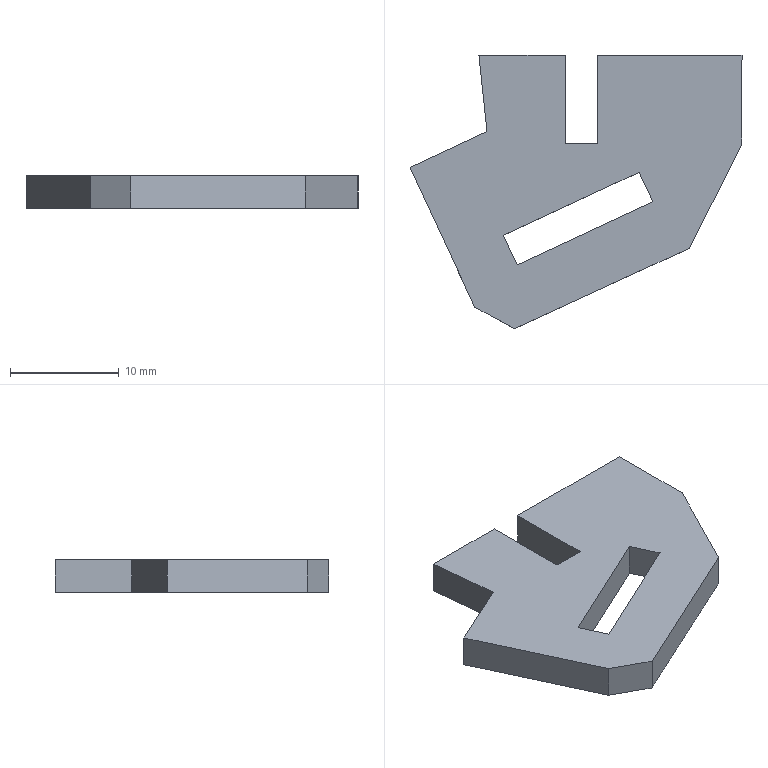Part | SolidWorks | features BaseBody 1 | 1 solid | 18 faces | box 30.485 x 25.117 x 3 mm | volume 1409 mm3 | plane 18
STEP:
#1=CARTESIAN_POINT('',(16.164,-13.547,-1.5));
#2=VERTEX_POINT('',#1);
#3=CARTESIAN_POINT('',(14.9,-10.831,-1.5));
#4=VERTEX_POINT('',#3);
#5=CARTESIAN_POINT('',(8.106,3.772,-1.5));
#6=DIRECTION('',(-0.4219,0.9067,0.));
#7=VECTOR('',#6,1000.);
#8=LINE('',#5,#7);
#9=EDGE_CURVE('',#2,#4,#8,.T.);
#10=ORIENTED_EDGE('',*,*,#9,.T.);
#11=CARTESIAN_POINT('',(2.431,-16.623,-1.5));
#12=VERTEX_POINT('',#11);
#13=CARTESIAN_POINT('',(6.783,-14.601,-1.5));
#14=DIRECTION('',(-0.9069,-0.4213,0.));
#15=VECTOR('',#14,1000.);
#16=LINE('',#13,#15);
#17=EDGE_CURVE('',#4,#12,#16,.T.);
#18=ORIENTED_EDGE('',*,*,#17,.T.);
#19=CARTESIAN_POINT('',(3.694,-19.34,-1.5));
#20=VERTEX_POINT('',#19);
#21=CARTESIAN_POINT('',(-4.353,-2.023,-1.5));
#22=DIRECTION('',(0.4214,-0.9069,0.));
#23=VECTOR('',#22,1000.);
#24=LINE('',#21,#23);
#25=EDGE_CURVE('',#12,#20,#24,.T.);
#26=ORIENTED_EDGE('',*,*,#25,.T.);
#27=CARTESIAN_POINT('',(8.045,-17.318,-1.5));
#28=DIRECTION('',(0.9069,0.4213,0.));
#29=VECTOR('',#28,1000.);
#30=LINE('',#27,#29);
#31=EDGE_CURVE('',#20,#2,#30,.T.);
#32=ORIENTED_EDGE('',*,*,#31,.T.);
#33=EDGE_LOOP('',(#10,#18,#26,#32));
#34=FACE_BOUND('',#33,.T.);
#35=CARTESIAN_POINT('',(19.491,-17.818,-1.5));
#36=VERTEX_POINT('',#35);
#37=CARTESIAN_POINT('',(24.349,-8.242,-1.5));
#38=VERTEX_POINT('',#37);
#39=CARTESIAN_POINT('',(22.69,-11.511,-1.5));
#40=DIRECTION('',(0.4524,0.8918,0.));
#41=VECTOR('',#40,1000.);
#42=LINE('',#39,#41);
#43=EDGE_CURVE('',#36,#38,#42,.T.);
#44=ORIENTED_EDGE('',*,*,#43,.F.);
#45=CARTESIAN_POINT('',(3.466,-25.2,-1.5));
#46=VERTEX_POINT('',#45);
#47=CARTESIAN_POINT('',(10.184,-22.105,-1.5));
#48=DIRECTION('',(0.9083,0.4184,0.));
#49=VECTOR('',#48,1000.);
#50=LINE('',#47,#49);
#51=EDGE_CURVE('',#46,#36,#50,.T.);
#52=ORIENTED_EDGE('',*,*,#51,.F.);
#53=CARTESIAN_POINT('',(-0.1829,-23.22,-1.5));
#54=VERTEX_POINT('',#53);
#55=CARTESIAN_POINT('',(-9.776,-18.014,-1.5));
#56=DIRECTION('',(0.8789,-0.477,0.));
#57=VECTOR('',#56,1000.);
#58=LINE('',#55,#57);
#59=EDGE_CURVE('',#54,#46,#58,.T.);
#60=ORIENTED_EDGE('',*,*,#59,.F.);
#61=CARTESIAN_POINT('',(-6.136,-10.378,-1.5));
#62=VERTEX_POINT('',#61);
#63=CARTESIAN_POINT('',(-9.011,-4.177,-1.5));
#64=DIRECTION('',(0.4206,-0.9073,0.));
#65=VECTOR('',#64,1000.);
#66=LINE('',#63,#65);
#67=EDGE_CURVE('',#62,#54,#66,.T.);
#68=ORIENTED_EDGE('',*,*,#67,.F.);
#69=CARTESIAN_POINT('',(0.9311,-7.102,-1.5));
#70=VERTEX_POINT('',#69);
#71=CARTESIAN_POINT('',(2.875,-6.201,-1.5));
#72=DIRECTION('',(-0.9073,-0.4206,0.));
#73=VECTOR('',#72,1000.);
#74=LINE('',#71,#73);
#75=EDGE_CURVE('',#70,#62,#74,.T.);
#76=ORIENTED_EDGE('',*,*,#75,.F.);
#77=CARTESIAN_POINT('',(0.193,-0.08325,-1.5));
#78=VERTEX_POINT('',#77);
#79=CARTESIAN_POINT('',(0.1822,0.01916,-1.5));
#80=DIRECTION('',(0.1046,-0.9945,0.));
#81=VECTOR('',#80,1000.);
#82=LINE('',#79,#81);
#83=EDGE_CURVE('',#78,#70,#82,.T.);
#84=ORIENTED_EDGE('',*,*,#83,.F.);
#85=CARTESIAN_POINT('',(8.101,-0.08325,-1.5));
#86=VERTEX_POINT('',#85);
#87=CARTESIAN_POINT('',(0.,-0.08325,-1.5));
#88=DIRECTION('',(1.,0.,0.));
#89=VECTOR('',#88,1000.);
#90=LINE('',#87,#89);
#91=EDGE_CURVE('',#78,#86,#90,.T.);
#92=ORIENTED_EDGE('',*,*,#91,.T.);
#93=CARTESIAN_POINT('',(8.13,-8.195,-1.5));
#94=VERTEX_POINT('',#93);
#95=CARTESIAN_POINT('',(8.101,0.02877,-1.5));
#96=DIRECTION('',(-0.003551,1.,0.));
#97=VECTOR('',#96,1000.);
#98=LINE('',#95,#97);
#99=EDGE_CURVE('',#94,#86,#98,.T.);
#100=ORIENTED_EDGE('',*,*,#99,.F.);
#101=CARTESIAN_POINT('',(11.126,-8.195,-1.5));
#102=VERTEX_POINT('',#101);
#103=CARTESIAN_POINT('',(0.,-8.195,-1.5));
#104=DIRECTION('',(-1.,0.,0.));
#105=VECTOR('',#104,1000.);
#106=LINE('',#103,#105);
#107=EDGE_CURVE('',#102,#94,#106,.T.);
#108=ORIENTED_EDGE('',*,*,#107,.F.);
#109=CARTESIAN_POINT('',(11.126,-0.08325,-1.5));
#110=VERTEX_POINT('',#109);
#111=CARTESIAN_POINT('',(11.126,0.,-1.5));
#112=DIRECTION('',(0.,-1.,0.));
#113=VECTOR('',#112,1000.);
#114=LINE('',#111,#113);
#115=EDGE_CURVE('',#110,#102,#114,.T.);
#116=ORIENTED_EDGE('',*,*,#115,.F.);
#117=CARTESIAN_POINT('',(24.349,-0.08325,-1.5));
#118=VERTEX_POINT('',#117);
#119=CARTESIAN_POINT('',(0.,-0.08325,-1.5));
#120=DIRECTION('',(1.,0.,0.));
#121=VECTOR('',#120,1000.);
#122=LINE('',#119,#121);
#123=EDGE_CURVE('',#110,#118,#122,.T.);
#124=ORIENTED_EDGE('',*,*,#123,.T.);
#125=CARTESIAN_POINT('',(24.349,0.,-1.5));
#126=DIRECTION('',(0.,1.,0.));
#127=VECTOR('',#126,1000.);
#128=LINE('',#125,#127);
#129=EDGE_CURVE('',#38,#118,#128,.T.);
#130=ORIENTED_EDGE('',*,*,#129,.F.);
#131=EDGE_LOOP('',(#44,#52,#60,#68,#76,#84,#92,#100,#108,#116,#124,#130));
#132=FACE_OUTER_BOUND('',#131,.T.);
#133=CARTESIAN_POINT('',(0.,0.,-1.5));
#134=DIRECTION('',(0.,0.,1.));
#135=DIRECTION('',(1.,0.,0.));
#136=AXIS2_PLACEMENT_3D('',#133,#134,#135);
#137=PLANE('',#136);
#138=ADVANCED_FACE('',(#34,#132),#137,.F.);
#139=CARTESIAN_POINT('',(16.164,-13.547,1.5));
#140=VERTEX_POINT('',#139);
#141=CARTESIAN_POINT('',(14.9,-10.831,1.5));
#142=VERTEX_POINT('',#141);
#143=CARTESIAN_POINT('',(8.106,3.772,1.5));
#144=DIRECTION('',(-0.4219,0.9067,0.));
#145=VECTOR('',#144,1000.);
#146=LINE('',#143,#145);
#147=EDGE_CURVE('',#140,#142,#146,.T.);
#148=ORIENTED_EDGE('',*,*,#147,.F.);
#149=CARTESIAN_POINT('',(3.694,-19.34,1.5));
#150=VERTEX_POINT('',#149);
#151=CARTESIAN_POINT('',(8.045,-17.318,1.5));
#152=DIRECTION('',(0.9069,0.4213,0.));
#153=VECTOR('',#152,1000.);
#154=LINE('',#151,#153);
#155=EDGE_CURVE('',#150,#140,#154,.T.);
#156=ORIENTED_EDGE('',*,*,#155,.F.);
#157=CARTESIAN_POINT('',(2.431,-16.623,1.5));
#158=VERTEX_POINT('',#157);
#159=CARTESIAN_POINT('',(-4.353,-2.023,1.5));
#160=DIRECTION('',(0.4214,-0.9069,0.));
#161=VECTOR('',#160,1000.);
#162=LINE('',#159,#161);
#163=EDGE_CURVE('',#158,#150,#162,.T.);
#164=ORIENTED_EDGE('',*,*,#163,.F.);
#165=CARTESIAN_POINT('',(6.783,-14.601,1.5));
#166=DIRECTION('',(-0.9069,-0.4213,0.));
#167=VECTOR('',#166,1000.);
#168=LINE('',#165,#167);
#169=EDGE_CURVE('',#142,#158,#168,.T.);
#170=ORIENTED_EDGE('',*,*,#169,.F.);
#171=EDGE_LOOP('',(#148,#156,#164,#170));
#172=FACE_BOUND('',#171,.T.);
#173=CARTESIAN_POINT('',(19.491,-17.818,1.5));
#174=VERTEX_POINT('',#173);
#175=CARTESIAN_POINT('',(24.349,-8.242,1.5));
#176=VERTEX_POINT('',#175);
#177=CARTESIAN_POINT('',(22.69,-11.511,1.5));
#178=DIRECTION('',(0.4524,0.8918,0.));
#179=VECTOR('',#178,1000.);
#180=LINE('',#177,#179);
#181=EDGE_CURVE('',#174,#176,#180,.T.);
#182=ORIENTED_EDGE('',*,*,#181,.T.);
#183=CARTESIAN_POINT('',(24.349,-0.08325,1.5));
#184=VERTEX_POINT('',#183);
#185=CARTESIAN_POINT('',(24.349,0.,1.5));
#186=DIRECTION('',(0.,1.,0.));
#187=VECTOR('',#186,1000.);
#188=LINE('',#185,#187);
#189=EDGE_CURVE('',#176,#184,#188,.T.);
#190=ORIENTED_EDGE('',*,*,#189,.T.);
#191=CARTESIAN_POINT('',(11.126,-0.08325,1.5));
#192=VERTEX_POINT('',#191);
#193=CARTESIAN_POINT('',(0.,-0.08325,1.5));
#194=DIRECTION('',(1.,0.,0.));
#195=VECTOR('',#194,1000.);
#196=LINE('',#193,#195);
#197=EDGE_CURVE('',#192,#184,#196,.T.);
#198=ORIENTED_EDGE('',*,*,#197,.F.);
#199=CARTESIAN_POINT('',(11.126,-8.195,1.5));
#200=VERTEX_POINT('',#199);
#201=CARTESIAN_POINT('',(11.126,0.,1.5));
#202=DIRECTION('',(0.,-1.,0.));
#203=VECTOR('',#202,1000.);
#204=LINE('',#201,#203);
#205=EDGE_CURVE('',#192,#200,#204,.T.);
#206=ORIENTED_EDGE('',*,*,#205,.T.);
#207=CARTESIAN_POINT('',(8.13,-8.195,1.5));
#208=VERTEX_POINT('',#207);
#209=CARTESIAN_POINT('',(0.,-8.195,1.5));
#210=DIRECTION('',(-1.,0.,0.));
#211=VECTOR('',#210,1000.);
#212=LINE('',#209,#211);
#213=EDGE_CURVE('',#200,#208,#212,.T.);
#214=ORIENTED_EDGE('',*,*,#213,.T.);
#215=CARTESIAN_POINT('',(8.101,-0.08325,1.5));
#216=VERTEX_POINT('',#215);
#217=CARTESIAN_POINT('',(8.101,0.02877,1.5));
#218=DIRECTION('',(-0.003551,1.,0.));
#219=VECTOR('',#218,1000.);
#220=LINE('',#217,#219);
#221=EDGE_CURVE('',#208,#216,#220,.T.);
#222=ORIENTED_EDGE('',*,*,#221,.T.);
#223=CARTESIAN_POINT('',(0.193,-0.08325,1.5));
#224=VERTEX_POINT('',#223);
#225=CARTESIAN_POINT('',(0.,-0.08325,1.5));
#226=DIRECTION('',(1.,0.,0.));
#227=VECTOR('',#226,1000.);
#228=LINE('',#225,#227);
#229=EDGE_CURVE('',#224,#216,#228,.T.);
#230=ORIENTED_EDGE('',*,*,#229,.F.);
#231=CARTESIAN_POINT('',(0.9311,-7.102,1.5));
#232=VERTEX_POINT('',#231);
#233=CARTESIAN_POINT('',(0.1822,0.01916,1.5));
#234=DIRECTION('',(0.1046,-0.9945,0.));
#235=VECTOR('',#234,1000.);
#236=LINE('',#233,#235);
#237=EDGE_CURVE('',#224,#232,#236,.T.);
#238=ORIENTED_EDGE('',*,*,#237,.T.);
#239=CARTESIAN_POINT('',(-6.136,-10.378,1.5));
#240=VERTEX_POINT('',#239);
#241=CARTESIAN_POINT('',(2.875,-6.201,1.5));
#242=DIRECTION('',(-0.9073,-0.4206,0.));
#243=VECTOR('',#242,1000.);
#244=LINE('',#241,#243);
#245=EDGE_CURVE('',#232,#240,#244,.T.);
#246=ORIENTED_EDGE('',*,*,#245,.T.);
#247=CARTESIAN_POINT('',(-0.1829,-23.22,1.5));
#248=VERTEX_POINT('',#247);
#249=CARTESIAN_POINT('',(-9.011,-4.177,1.5));
#250=DIRECTION('',(0.4206,-0.9073,0.));
#251=VECTOR('',#250,1000.);
#252=LINE('',#249,#251);
#253=EDGE_CURVE('',#240,#248,#252,.T.);
#254=ORIENTED_EDGE('',*,*,#253,.T.);
#255=CARTESIAN_POINT('',(3.466,-25.2,1.5));
#256=VERTEX_POINT('',#255);
#257=CARTESIAN_POINT('',(-9.776,-18.014,1.5));
#258=DIRECTION('',(0.8789,-0.477,0.));
#259=VECTOR('',#258,1000.);
#260=LINE('',#257,#259);
#261=EDGE_CURVE('',#248,#256,#260,.T.);
#262=ORIENTED_EDGE('',*,*,#261,.T.);
#263=CARTESIAN_POINT('',(10.184,-22.105,1.5));
#264=DIRECTION('',(0.9083,0.4184,0.));
#265=VECTOR('',#264,1000.);
#266=LINE('',#263,#265);
#267=EDGE_CURVE('',#256,#174,#266,.T.);
#268=ORIENTED_EDGE('',*,*,#267,.T.);
#269=EDGE_LOOP('',(#182,#190,#198,#206,#214,#222,#230,#238,#246,#254,#262,#268));
#270=FACE_OUTER_BOUND('',#269,.T.);
#271=CARTESIAN_POINT('',(0.,0.,1.5));
#272=DIRECTION('',(0.,0.,1.));
#273=DIRECTION('',(1.,0.,0.));
#274=AXIS2_PLACEMENT_3D('',#271,#272,#273);
#275=PLANE('',#274);
#276=ADVANCED_FACE('',(#172,#270),#275,.T.);
#277=ORIENTED_EDGE('',*,*,#51,.T.);
#278=CARTESIAN_POINT('',(19.491,-17.818,1.5));
#279=DIRECTION('',(0.,0.,-1.));
#280=VECTOR('',#279,1000.);
#281=LINE('',#278,#280);
#282=EDGE_CURVE('',#174,#36,#281,.T.);
#283=ORIENTED_EDGE('',*,*,#282,.F.);
#284=ORIENTED_EDGE('',*,*,#267,.F.);
#285=CARTESIAN_POINT('',(3.466,-25.2,1.5));
#286=DIRECTION('',(0.,0.,-1.));
#287=VECTOR('',#286,1000.);
#288=LINE('',#285,#287);
#289=EDGE_CURVE('',#256,#46,#288,.T.);
#290=ORIENTED_EDGE('',*,*,#289,.T.);
#291=EDGE_LOOP('',(#277,#283,#284,#290));
#292=FACE_OUTER_BOUND('',#291,.T.);
#293=CARTESIAN_POINT('',(10.184,-22.105,1.5));
#294=DIRECTION('',(-0.4184,0.9083,0.));
#295=DIRECTION('',(0.,0.,1.));
#296=AXIS2_PLACEMENT_3D('',#293,#294,#295);
#297=PLANE('',#296);
#298=ADVANCED_FACE('',(#292),#297,.F.);
#299=ORIENTED_EDGE('',*,*,#17,.F.);
#300=CARTESIAN_POINT('',(14.9,-10.831,1.5));
#301=DIRECTION('',(0.,0.,-1.));
#302=VECTOR('',#301,1000.);
#303=LINE('',#300,#302);
#304=EDGE_CURVE('',#142,#4,#303,.T.);
#305=ORIENTED_EDGE('',*,*,#304,.F.);
#306=ORIENTED_EDGE('',*,*,#169,.T.);
#307=CARTESIAN_POINT('',(2.431,-16.623,1.5));
#308=DIRECTION('',(0.,0.,-1.));
#309=VECTOR('',#308,1000.);
#310=LINE('',#307,#309);
#311=EDGE_CURVE('',#158,#12,#310,.T.);
#312=ORIENTED_EDGE('',*,*,#311,.T.);
#313=EDGE_LOOP('',(#299,#305,#306,#312));
#314=FACE_OUTER_BOUND('',#313,.T.);
#315=CARTESIAN_POINT('',(6.783,-14.601,1.5));
#316=DIRECTION('',(0.4213,-0.9069,0.));
#317=DIRECTION('',(0.,0.,-1.));
#318=AXIS2_PLACEMENT_3D('',#315,#316,#317);
#319=PLANE('',#318);
#320=ADVANCED_FACE('',(#314),#319,.T.);
#321=ORIENTED_EDGE('',*,*,#25,.F.);
#322=ORIENTED_EDGE('',*,*,#311,.F.);
#323=ORIENTED_EDGE('',*,*,#163,.T.);
#324=CARTESIAN_POINT('',(3.694,-19.34,1.5));
#325=DIRECTION('',(0.,0.,-1.));
#326=VECTOR('',#325,1000.);
#327=LINE('',#324,#326);
#328=EDGE_CURVE('',#150,#20,#327,.T.);
#329=ORIENTED_EDGE('',*,*,#328,.T.);
#330=EDGE_LOOP('',(#321,#322,#323,#329));
#331=FACE_OUTER_BOUND('',#330,.T.);
#332=CARTESIAN_POINT('',(-4.353,-2.023,1.5));
#333=DIRECTION('',(0.9069,0.4214,0.));
#334=DIRECTION('',(0.,0.,-1.));
#335=AXIS2_PLACEMENT_3D('',#332,#333,#334);
#336=PLANE('',#335);
#337=ADVANCED_FACE('',(#331),#336,.T.);
#338=ORIENTED_EDGE('',*,*,#31,.F.);
#339=ORIENTED_EDGE('',*,*,#328,.F.);
#340=ORIENTED_EDGE('',*,*,#155,.T.);
#341=CARTESIAN_POINT('',(16.164,-13.547,1.5));
#342=DIRECTION('',(0.,0.,-1.));
#343=VECTOR('',#342,1000.);
#344=LINE('',#341,#343);
#345=EDGE_CURVE('',#140,#2,#344,.T.);
#346=ORIENTED_EDGE('',*,*,#345,.T.);
#347=EDGE_LOOP('',(#338,#339,#340,#346));
#348=FACE_OUTER_BOUND('',#347,.T.);
#349=CARTESIAN_POINT('',(8.045,-17.318,1.5));
#350=DIRECTION('',(-0.4213,0.9069,0.));
#351=DIRECTION('',(0.,0.,1.));
#352=AXIS2_PLACEMENT_3D('',#349,#350,#351);
#353=PLANE('',#352);
#354=ADVANCED_FACE('',(#348),#353,.T.);
#355=ORIENTED_EDGE('',*,*,#9,.F.);
#356=ORIENTED_EDGE('',*,*,#345,.F.);
#357=ORIENTED_EDGE('',*,*,#147,.T.);
#358=ORIENTED_EDGE('',*,*,#304,.T.);
#359=EDGE_LOOP('',(#355,#356,#357,#358));
#360=FACE_OUTER_BOUND('',#359,.T.);
#361=CARTESIAN_POINT('',(8.106,3.772,1.5));
#362=DIRECTION('',(-0.9067,-0.4219,0.));
#363=DIRECTION('',(-0.4219,0.9067,0.));
#364=AXIS2_PLACEMENT_3D('',#361,#362,#363);
#365=PLANE('',#364);
#366=ADVANCED_FACE('',(#360),#365,.T.);
#367=ORIENTED_EDGE('',*,*,#59,.T.);
#368=ORIENTED_EDGE('',*,*,#289,.F.);
#369=ORIENTED_EDGE('',*,*,#261,.F.);
#370=CARTESIAN_POINT('',(-0.1829,-23.22,1.5));
#371=DIRECTION('',(0.,0.,-1.));
#372=VECTOR('',#371,1000.);
#373=LINE('',#370,#372);
#374=EDGE_CURVE('',#248,#54,#373,.T.);
#375=ORIENTED_EDGE('',*,*,#374,.T.);
#376=EDGE_LOOP('',(#367,#368,#369,#375));
#377=FACE_OUTER_BOUND('',#376,.T.);
#378=CARTESIAN_POINT('',(-9.776,-18.014,1.5));
#379=DIRECTION('',(0.477,0.8789,0.));
#380=DIRECTION('',(0.,0.,-1.));
#381=AXIS2_PLACEMENT_3D('',#378,#379,#380);
#382=PLANE('',#381);
#383=ADVANCED_FACE('',(#377),#382,.F.);
#384=ORIENTED_EDGE('',*,*,#67,.T.);
#385=ORIENTED_EDGE('',*,*,#374,.F.);
#386=ORIENTED_EDGE('',*,*,#253,.F.);
#387=CARTESIAN_POINT('',(-6.136,-10.378,1.5));
#388=DIRECTION('',(0.,0.,-1.));
#389=VECTOR('',#388,1000.);
#390=LINE('',#387,#389);
#391=EDGE_CURVE('',#240,#62,#390,.T.);
#392=ORIENTED_EDGE('',*,*,#391,.T.);
#393=EDGE_LOOP('',(#384,#385,#386,#392));
#394=FACE_OUTER_BOUND('',#393,.T.);
#395=CARTESIAN_POINT('',(-9.011,-4.177,1.5));
#396=DIRECTION('',(0.9073,0.4206,0.));
#397=DIRECTION('',(0.,0.,-1.));
#398=AXIS2_PLACEMENT_3D('',#395,#396,#397);
#399=PLANE('',#398);
#400=ADVANCED_FACE('',(#394),#399,.F.);
#401=ORIENTED_EDGE('',*,*,#75,.T.);
#402=ORIENTED_EDGE('',*,*,#391,.F.);
#403=ORIENTED_EDGE('',*,*,#245,.F.);
#404=CARTESIAN_POINT('',(0.9311,-7.102,1.5));
#405=DIRECTION('',(0.,0.,-1.));
#406=VECTOR('',#405,1000.);
#407=LINE('',#404,#406);
#408=EDGE_CURVE('',#232,#70,#407,.T.);
#409=ORIENTED_EDGE('',*,*,#408,.T.);
#410=EDGE_LOOP('',(#401,#402,#403,#409));
#411=FACE_OUTER_BOUND('',#410,.T.);
#412=CARTESIAN_POINT('',(2.875,-6.201,1.5));
#413=DIRECTION('',(0.4206,-0.9073,0.));
#414=DIRECTION('',(0.,0.,-1.));
#415=AXIS2_PLACEMENT_3D('',#412,#413,#414);
#416=PLANE('',#415);
#417=ADVANCED_FACE('',(#411),#416,.F.);
#418=ORIENTED_EDGE('',*,*,#83,.T.);
#419=ORIENTED_EDGE('',*,*,#408,.F.);
#420=ORIENTED_EDGE('',*,*,#237,.F.);
#421=CARTESIAN_POINT('',(0.193,-0.08325,1.5));
#422=DIRECTION('',(0.,0.,-1.));
#423=VECTOR('',#422,1000.);
#424=LINE('',#421,#423);
#425=EDGE_CURVE('',#224,#78,#424,.T.);
#426=ORIENTED_EDGE('',*,*,#425,.T.);
#427=EDGE_LOOP('',(#418,#419,#420,#426));
#428=FACE_OUTER_BOUND('',#427,.T.);
#429=CARTESIAN_POINT('',(0.1822,0.01916,1.5));
#430=DIRECTION('',(0.9945,0.1046,0.));
#431=DIRECTION('',(0.,0.,-1.));
#432=AXIS2_PLACEMENT_3D('',#429,#430,#431);
#433=PLANE('',#432);
#434=ADVANCED_FACE('',(#428),#433,.F.);
#435=ORIENTED_EDGE('',*,*,#91,.F.);
#436=ORIENTED_EDGE('',*,*,#425,.F.);
#437=ORIENTED_EDGE('',*,*,#229,.T.);
#438=CARTESIAN_POINT('',(8.101,-0.08325,1.5));
#439=DIRECTION('',(0.,0.,-1.));
#440=VECTOR('',#439,1000.);
#441=LINE('',#438,#440);
#442=EDGE_CURVE('',#216,#86,#441,.T.);
#443=ORIENTED_EDGE('',*,*,#442,.T.);
#444=EDGE_LOOP('',(#435,#436,#437,#443));
#445=FACE_OUTER_BOUND('',#444,.T.);
#446=CARTESIAN_POINT('',(0.,-0.08325,1.5));
#447=DIRECTION('',(0.,1.,0.));
#448=DIRECTION('',(1.,0.,0.));
#449=AXIS2_PLACEMENT_3D('',#446,#447,#448);
#450=PLANE('',#449);
#451=ADVANCED_FACE('',(#445),#450,.T.);
#452=ORIENTED_EDGE('',*,*,#99,.T.);
#453=ORIENTED_EDGE('',*,*,#442,.F.);
#454=ORIENTED_EDGE('',*,*,#221,.F.);
#455=CARTESIAN_POINT('',(8.13,-8.195,1.5));
#456=DIRECTION('',(0.,0.,-1.));
#457=VECTOR('',#456,1000.);
#458=LINE('',#455,#457);
#459=EDGE_CURVE('',#208,#94,#458,.T.);
#460=ORIENTED_EDGE('',*,*,#459,.T.);
#461=EDGE_LOOP('',(#452,#453,#454,#460));
#462=FACE_OUTER_BOUND('',#461,.T.);
#463=CARTESIAN_POINT('',(8.101,0.02877,1.5));
#464=DIRECTION('',(-1.,-0.003551,0.));
#465=DIRECTION('',(-0.003551,1.,0.));
#466=AXIS2_PLACEMENT_3D('',#463,#464,#465);
#467=PLANE('',#466);
#468=ADVANCED_FACE('',(#462),#467,.F.);
#469=ORIENTED_EDGE('',*,*,#107,.T.);
#470=ORIENTED_EDGE('',*,*,#459,.F.);
#471=ORIENTED_EDGE('',*,*,#213,.F.);
#472=CARTESIAN_POINT('',(11.126,-8.195,1.5));
#473=DIRECTION('',(0.,0.,-1.));
#474=VECTOR('',#473,1000.);
#475=LINE('',#472,#474);
#476=EDGE_CURVE('',#200,#102,#475,.T.);
#477=ORIENTED_EDGE('',*,*,#476,.T.);
#478=EDGE_LOOP('',(#469,#470,#471,#477));
#479=FACE_OUTER_BOUND('',#478,.T.);
#480=CARTESIAN_POINT('',(0.,-8.195,1.5));
#481=DIRECTION('',(0.,-1.,0.));
#482=DIRECTION('',(0.,0.,-1.));
#483=AXIS2_PLACEMENT_3D('',#480,#481,#482);
#484=PLANE('',#483);
#485=ADVANCED_FACE('',(#479),#484,.F.);
#486=ORIENTED_EDGE('',*,*,#115,.T.);
#487=ORIENTED_EDGE('',*,*,#476,.F.);
#488=ORIENTED_EDGE('',*,*,#205,.F.);
#489=CARTESIAN_POINT('',(11.126,-0.08325,1.5));
#490=DIRECTION('',(0.,0.,-1.));
#491=VECTOR('',#490,1000.);
#492=LINE('',#489,#491);
#493=EDGE_CURVE('',#192,#110,#492,.T.);
#494=ORIENTED_EDGE('',*,*,#493,.T.);
#495=EDGE_LOOP('',(#486,#487,#488,#494));
#496=FACE_OUTER_BOUND('',#495,.T.);
#497=CARTESIAN_POINT('',(11.126,0.,1.5));
#498=DIRECTION('',(1.,0.,0.));
#499=DIRECTION('',(0.,1.,0.));
#500=AXIS2_PLACEMENT_3D('',#497,#498,#499);
#501=PLANE('',#500);
#502=ADVANCED_FACE('',(#496),#501,.F.);
#503=ORIENTED_EDGE('',*,*,#123,.F.);
#504=ORIENTED_EDGE('',*,*,#493,.F.);
#505=ORIENTED_EDGE('',*,*,#197,.T.);
#506=CARTESIAN_POINT('',(24.349,-0.08325,1.5));
#507=DIRECTION('',(0.,0.,-1.));
#508=VECTOR('',#507,1000.);
#509=LINE('',#506,#508);
#510=EDGE_CURVE('',#184,#118,#509,.T.);
#511=ORIENTED_EDGE('',*,*,#510,.T.);
#512=EDGE_LOOP('',(#503,#504,#505,#511));
#513=FACE_OUTER_BOUND('',#512,.T.);
#514=CARTESIAN_POINT('',(0.,-0.08325,1.5));
#515=DIRECTION('',(0.,1.,0.));
#516=DIRECTION('',(1.,0.,0.));
#517=AXIS2_PLACEMENT_3D('',#514,#515,#516);
#518=PLANE('',#517);
#519=ADVANCED_FACE('',(#513),#518,.T.);
#520=ORIENTED_EDGE('',*,*,#129,.T.);
#521=ORIENTED_EDGE('',*,*,#510,.F.);
#522=ORIENTED_EDGE('',*,*,#189,.F.);
#523=CARTESIAN_POINT('',(24.349,-8.242,1.5));
#524=DIRECTION('',(0.,0.,-1.));
#525=VECTOR('',#524,1000.);
#526=LINE('',#523,#525);
#527=EDGE_CURVE('',#176,#38,#526,.T.);
#528=ORIENTED_EDGE('',*,*,#527,.T.);
#529=EDGE_LOOP('',(#520,#521,#522,#528));
#530=FACE_OUTER_BOUND('',#529,.T.);
#531=CARTESIAN_POINT('',(24.349,0.,1.5));
#532=DIRECTION('',(-1.,0.,0.));
#533=DIRECTION('',(0.,0.,1.));
#534=AXIS2_PLACEMENT_3D('',#531,#532,#533);
#535=PLANE('',#534);
#536=ADVANCED_FACE('',(#530),#535,.F.);
#537=ORIENTED_EDGE('',*,*,#43,.T.);
#538=ORIENTED_EDGE('',*,*,#527,.F.);
#539=ORIENTED_EDGE('',*,*,#181,.F.);
#540=ORIENTED_EDGE('',*,*,#282,.T.);
#541=EDGE_LOOP('',(#537,#538,#539,#540));
#542=FACE_OUTER_BOUND('',#541,.T.);
#543=CARTESIAN_POINT('',(22.69,-11.511,1.5));
#544=DIRECTION('',(-0.8918,0.4524,0.));
#545=DIRECTION('',(0.,0.,1.));
#546=AXIS2_PLACEMENT_3D('',#543,#544,#545);
#547=PLANE('',#546);
#548=ADVANCED_FACE('',(#542),#547,.F.);
#549=CLOSED_SHELL('',(#138,#276,#298,#320,#337,#354,#366,#383,#400,#417,#434,#451,#468,#485,#502,#519,#536,#548));
#550=MANIFOLD_SOLID_BREP('',#549);
#551=CARTESIAN_POINT('',(0.,0.,0.));
#552=DIRECTION('',(0.,0.,1.));
#553=DIRECTION('',(1.,0.,0.));
#554=AXIS2_PLACEMENT_3D('',#551,#552,#553);
#555=(LENGTH_UNIT()NAMED_UNIT(*)SI_UNIT(.MILLI.,.METRE.));
#556=UNCERTAINTY_MEASURE_WITH_UNIT(LENGTH_MEASURE(0.00001),#555,'','');
#557=(NAMED_UNIT(*)PLANE_ANGLE_UNIT()SI_UNIT($,.RADIAN.));
#558=(NAMED_UNIT(*)SI_UNIT($,.STERADIAN.)SOLID_ANGLE_UNIT());
#559=(GEOMETRIC_REPRESENTATION_CONTEXT(3)GLOBAL_UNCERTAINTY_ASSIGNED_CONTEXT((#556))GLOBAL_UNIT_ASSIGNED_CONTEXT((#555,#557,#558))REPRESENTATION_CONTEXT('',''));
#560=ADVANCED_BREP_SHAPE_REPRESENTATION('',(#550,#554),#559);